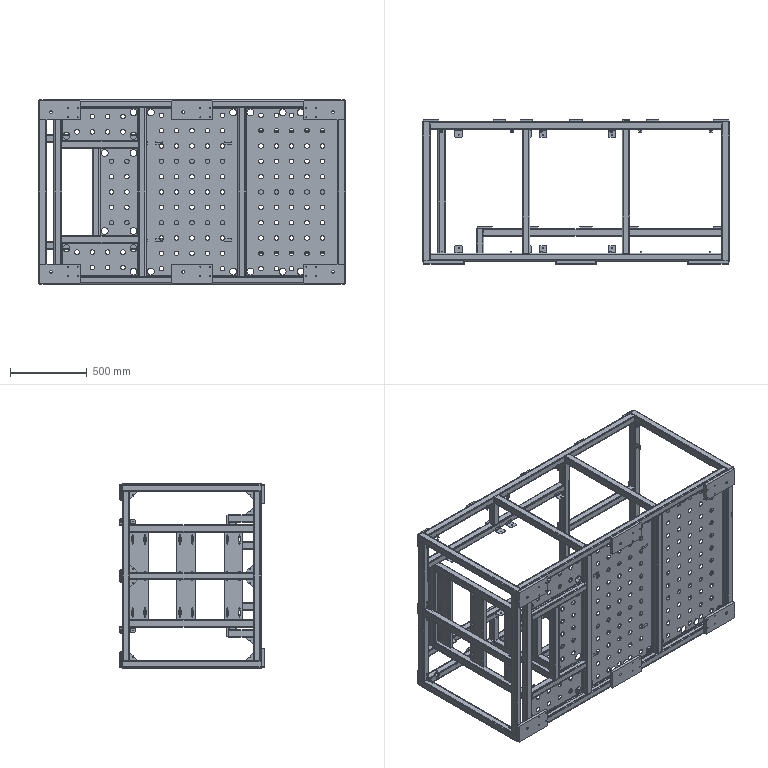Part | NX | 130 solids | 2609 faces | box 2000 x 940 x 1200 mm | volume 45255626 mm3 | plane 1745 | cylinder 844 | cone 20 | commonest cylinder face diameters 4 x180 14 x180 30 x136 8.5 x61 5 x44 9 x36